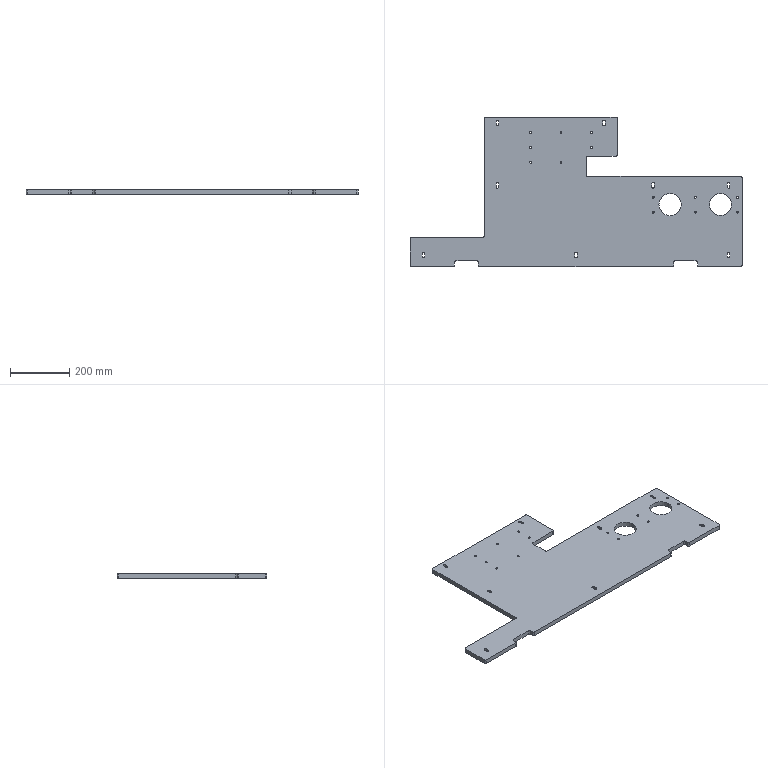Part | STEP file | PN_0001 | 1 solid | 140 faces | box 1120 x 505 x 15 mm | volume 5379555 mm3 | cylinder 80 | plane 60 | commonest cylinder face diameters 6.8 x22 10 x18 9 x16 15 x16 6 x4 75 x4